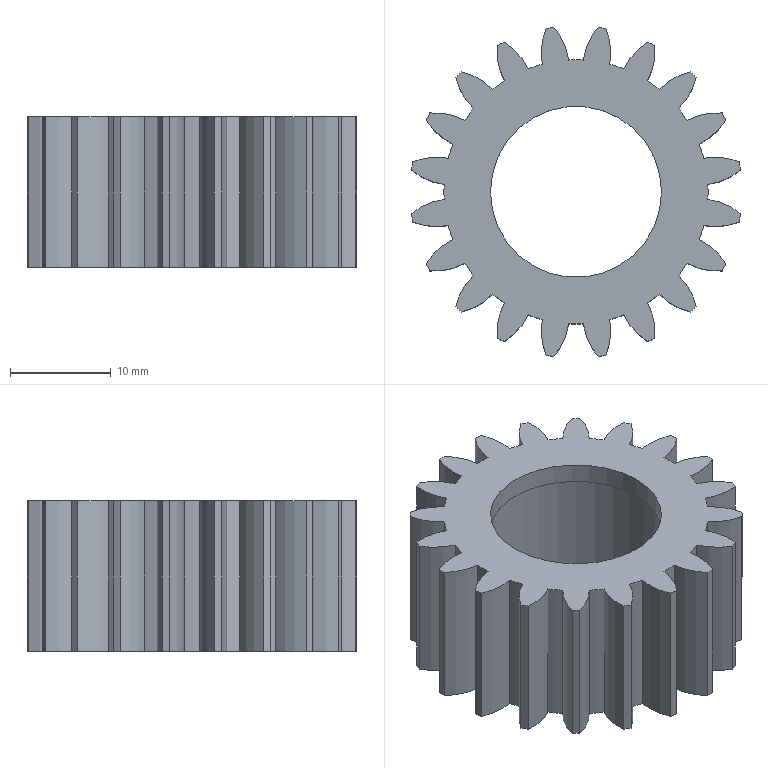Part | NX | features BREP 1 | 1 solid | 89 faces | box 32.708 x 32.708 x 15 mm | volume 6056 mm3 | cylinder 84 | plane 5 | commonest cylinder face diameters 12 x40 26.248 x20 33 x20 19 x2 17 x1 20 x1